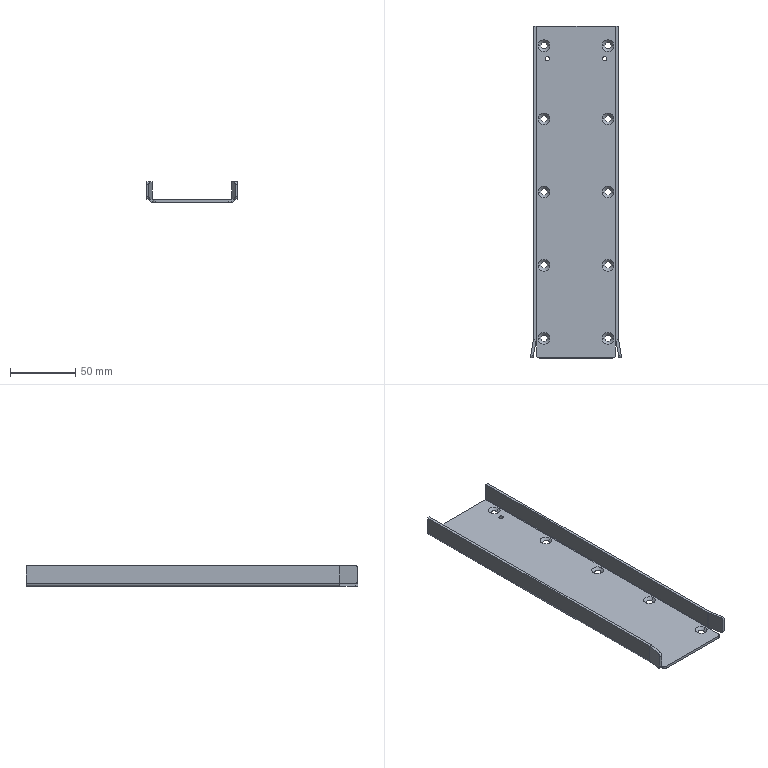Part | SolidWorks | features EdgeFlange 2, HoleWzd 2, Fillet 1, FlatPattern 1, ICE 1, SMBaseFlange 1, SheetMetal 1 | 1 solid | 70 faces | box 69.801 x 254 x 16 mm | volume 45736 mm3 | plane 32 | cone 20 | cylinder 18 | commonest cylinder face diameters 4 x6 0.6 x4 3.3 x4 4.6 x4